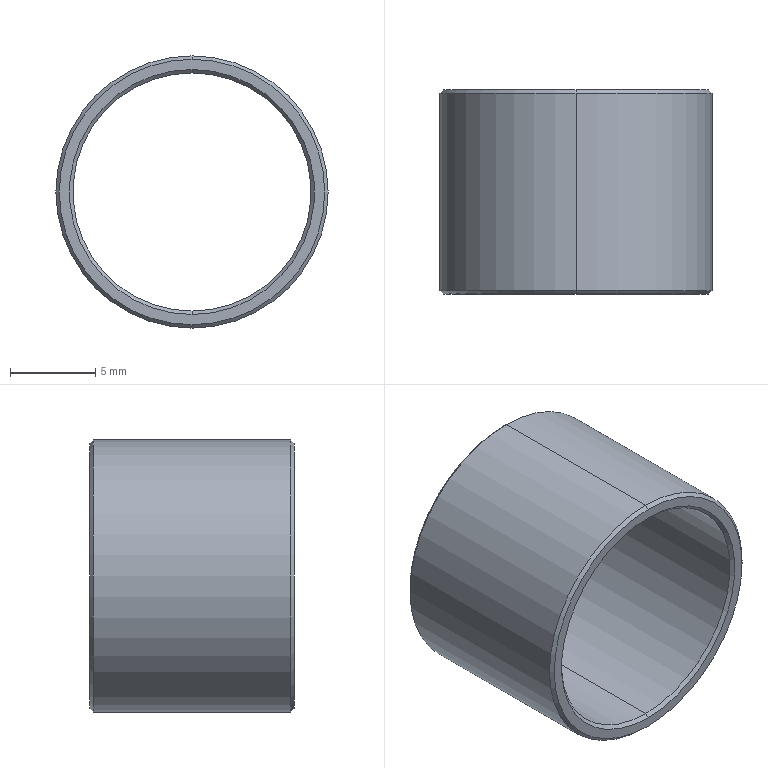Part | STEP file | Lead screw shaft end spacer V1.201001 | 1 solid | 14 faces | box 16 x 12 x 16 mm | volume 561.717 mm3 | cone 8 | cylinder 4 | plane 2 | commonest cylinder face diameters 14 x2 16 x2
STEP:
#1=CARTESIAN_POINT('',(0.,0.,0.));
#2=DIRECTION('',(0.,0.,1.));
#3=DIRECTION('',(1.,0.,0.));
#4=AXIS2_PLACEMENT_3D('',#1,#2,#3);
#5=CARTESIAN_POINT('',(0.,11.8,7.));
#6=VERTEX_POINT('',#5);
#7=CARTESIAN_POINT('',(0.,12.,7.2));
#8=VERTEX_POINT('',#7);
#9=CARTESIAN_POINT('',(0.,11.8,7.));
#10=DIRECTION('',(0.,0.7071,0.7071));
#11=VECTOR('',#10,1.);
#12=LINE('',#9,#11);
#13=CARTESIAN_POINT('',(0.,11.8,0.));
#14=DIRECTION('',(0.,1.,0.));
#15=DIRECTION('',(0.,0.,1.));
#16=AXIS2_PLACEMENT_3D('',#13,#14,#15);
#17=CONICAL_SURFACE('',#16,7.,0.7854);
#18=CARTESIAN_POINT('',(6.283,0.));
#19=DIRECTION('',(0.,1.));
#20=VECTOR('',#19,1.);
#21=LINE('',#18,#20);
#22=(GEOMETRIC_REPRESENTATION_CONTEXT(2)PARAMETRIC_REPRESENTATION_CONTEXT()REPRESENTATION_CONTEXT('',''));
#23=DEFINITIONAL_REPRESENTATION('',(#21),#22);
#24=PCURVE('',#17,#23);
#25=CARTESIAN_POINT('',(0.,11.8,0.));
#26=DIRECTION('',(0.,1.,0.));
#27=DIRECTION('',(0.,0.,1.));
#28=AXIS2_PLACEMENT_3D('',#25,#26,#27);
#29=CONICAL_SURFACE('',#28,7.,0.7854);
#30=CARTESIAN_POINT('',(0.,0.));
#31=DIRECTION('',(0.,1.));
#32=VECTOR('',#31,1.);
#33=LINE('',#30,#32);
#34=(GEOMETRIC_REPRESENTATION_CONTEXT(2)PARAMETRIC_REPRESENTATION_CONTEXT()REPRESENTATION_CONTEXT('',''));
#35=DEFINITIONAL_REPRESENTATION('',(#33),#34);
#36=PCURVE('',#29,#35);
#37=SURFACE_CURVE('',#12,(#24,#36),.PCURVE_S1.);
#38=EDGE_CURVE('',#6,#8,#37,.T.);
#39=ORIENTED_EDGE('',*,*,#38,.T.);
#40=CARTESIAN_POINT('',(0.,12.,-7.2));
#41=VERTEX_POINT('',#40);
#42=CARTESIAN_POINT('',(0.,12.,0.));
#43=DIRECTION('',(0.,-1.,0.));
#44=DIRECTION('',(0.,0.,1.));
#45=AXIS2_PLACEMENT_3D('',#42,#43,#44);
#46=CIRCLE('',#45,7.2);
#47=CARTESIAN_POINT('',(6.283,0.2));
#48=DIRECTION('',(-1.,0.));
#49=VECTOR('',#48,1.);
#50=LINE('',#47,#49);
#51=(GEOMETRIC_REPRESENTATION_CONTEXT(2)PARAMETRIC_REPRESENTATION_CONTEXT()REPRESENTATION_CONTEXT('',''));
#52=DEFINITIONAL_REPRESENTATION('',(#50),#51);
#53=PCURVE('',#17,#52);
#54=CARTESIAN_POINT('',(0.,12.,0.));
#55=DIRECTION('',(0.,1.,0.));
#56=DIRECTION('',(0.,0.,1.));
#57=AXIS2_PLACEMENT_3D('',#54,#55,#56);
#58=PLANE('',#57);
#59=CARTESIAN_POINT('',(7.2,0.));
#60=CARTESIAN_POINT('',(7.2,-12.471));
#61=CARTESIAN_POINT('',(-3.6,-6.235));
#62=CARTESIAN_POINT('',(-14.4,0.));
#63=CARTESIAN_POINT('',(-3.6,6.235));
#64=CARTESIAN_POINT('',(7.2,12.471));
#65=CARTESIAN_POINT('',(7.2,0.));
#66=(BOUNDED_CURVE()B_SPLINE_CURVE(2,(#59,#60,#61,#62,#63,#64,#65),.UNSPECIFIED.,.T.,.F.)B_SPLINE_CURVE_WITH_KNOTS((1,2,2,2,2,1),(-2.094,0.,2.094,4.189,6.283,8.378),.UNSPECIFIED.)CURVE()GEOMETRIC_REPRESENTATION_ITEM()RATIONAL_B_SPLINE_CURVE((1.,0.5,1.,0.5,1.,0.5,1.))REPRESENTATION_ITEM(''));
#67=(GEOMETRIC_REPRESENTATION_CONTEXT(2)PARAMETRIC_REPRESENTATION_CONTEXT()REPRESENTATION_CONTEXT('',''));
#68=DEFINITIONAL_REPRESENTATION('',(#66),#67);
#69=PCURVE('',#58,#68);
#70=SURFACE_CURVE('',#46,(#53,#69),.PCURVE_S1.);
#71=EDGE_CURVE('',#8,#41,#70,.T.);
#72=ORIENTED_EDGE('',*,*,#71,.T.);
#73=CARTESIAN_POINT('',(0.,11.8,-7.));
#74=VERTEX_POINT('',#73);
#75=CARTESIAN_POINT('',(0.,11.8,-7.));
#76=DIRECTION('',(0.,0.7071,-0.7071));
#77=VECTOR('',#76,1.);
#78=LINE('',#75,#77);
#79=CARTESIAN_POINT('',(3.142,0.));
#80=DIRECTION('',(0.,1.));
#81=VECTOR('',#80,1.);
#82=LINE('',#79,#81);
#83=(GEOMETRIC_REPRESENTATION_CONTEXT(2)PARAMETRIC_REPRESENTATION_CONTEXT()REPRESENTATION_CONTEXT('',''));
#84=DEFINITIONAL_REPRESENTATION('',(#82),#83);
#85=PCURVE('',#17,#84);
#86=CARTESIAN_POINT('',(3.142,0.));
#87=DIRECTION('',(0.,1.));
#88=VECTOR('',#87,1.);
#89=LINE('',#86,#88);
#90=(GEOMETRIC_REPRESENTATION_CONTEXT(2)PARAMETRIC_REPRESENTATION_CONTEXT()REPRESENTATION_CONTEXT('',''));
#91=DEFINITIONAL_REPRESENTATION('',(#89),#90);
#92=PCURVE('',#29,#91);
#93=SURFACE_CURVE('',#78,(#85,#92),.PCURVE_S1.);
#94=EDGE_CURVE('',#74,#41,#93,.T.);
#95=ORIENTED_EDGE('',*,*,#94,.F.);
#96=CARTESIAN_POINT('',(0.,11.8,0.));
#97=DIRECTION('',(0.,1.,0.));
#98=DIRECTION('',(0.,0.,1.));
#99=AXIS2_PLACEMENT_3D('',#96,#97,#98);
#100=CIRCLE('',#99,7.);
#101=CARTESIAN_POINT('',(0.,0.));
#102=DIRECTION('',(1.,0.));
#103=VECTOR('',#102,1.);
#104=LINE('',#101,#103);
#105=(GEOMETRIC_REPRESENTATION_CONTEXT(2)PARAMETRIC_REPRESENTATION_CONTEXT()REPRESENTATION_CONTEXT('',''));
#106=DEFINITIONAL_REPRESENTATION('',(#104),#105);
#107=PCURVE('',#17,#106);
#108=CARTESIAN_POINT('',(0.,12.,0.));
#109=DIRECTION('',(0.,-1.,0.));
#110=DIRECTION('',(0.,0.,-1.));
#111=AXIS2_PLACEMENT_3D('',#108,#109,#110);
#112=CYLINDRICAL_SURFACE('',#111,7.);
#113=CARTESIAN_POINT('',(9.425,0.2));
#114=DIRECTION('',(-1.,0.));
#115=VECTOR('',#114,1.);
#116=LINE('',#113,#115);
#117=(GEOMETRIC_REPRESENTATION_CONTEXT(2)PARAMETRIC_REPRESENTATION_CONTEXT()REPRESENTATION_CONTEXT('',''));
#118=DEFINITIONAL_REPRESENTATION('',(#116),#117);
#119=PCURVE('',#112,#118);
#120=SURFACE_CURVE('',#100,(#107,#119),.PCURVE_S1.);
#121=EDGE_CURVE('',#74,#6,#120,.T.);
#122=ORIENTED_EDGE('',*,*,#121,.T.);
#123=EDGE_LOOP('',(#39,#72,#95,#122));
#124=FACE_BOUND('',#123,.F.);
#125=ADVANCED_FACE('',(#124),#17,.F.);
#126=CARTESIAN_POINT('',(0.,12.,7.8));
#127=VERTEX_POINT('',#126);
#128=CARTESIAN_POINT('',(0.,12.,-7.8));
#129=VERTEX_POINT('',#128);
#130=CARTESIAN_POINT('',(0.,12.,0.));
#131=DIRECTION('',(0.,1.,0.));
#132=DIRECTION('',(0.,0.,1.));
#133=AXIS2_PLACEMENT_3D('',#130,#131,#132);
#134=CIRCLE('',#133,7.8);
#135=CARTESIAN_POINT('',(0.,12.,0.));
#136=DIRECTION('',(0.,-1.,0.));
#137=DIRECTION('',(0.,0.,-1.));
#138=AXIS2_PLACEMENT_3D('',#135,#136,#137);
#139=CONICAL_SURFACE('',#138,7.8,0.7854);
#140=CARTESIAN_POINT('',(3.142,0.));
#141=DIRECTION('',(-1.,0.));
#142=VECTOR('',#141,1.);
#143=LINE('',#140,#142);
#144=(GEOMETRIC_REPRESENTATION_CONTEXT(2)PARAMETRIC_REPRESENTATION_CONTEXT()REPRESENTATION_CONTEXT('',''));
#145=DEFINITIONAL_REPRESENTATION('',(#143),#144);
#146=PCURVE('',#139,#145);
#147=CARTESIAN_POINT('',(0.,0.));
#148=DIRECTION('',(1.,0.));
#149=AXIS2_PLACEMENT_2D('',#147,#148);
#150=CIRCLE('',#149,7.8);
#151=(GEOMETRIC_REPRESENTATION_CONTEXT(2)PARAMETRIC_REPRESENTATION_CONTEXT()REPRESENTATION_CONTEXT('',''));
#152=DEFINITIONAL_REPRESENTATION('',(#150),#151);
#153=PCURVE('',#58,#152);
#154=SURFACE_CURVE('',#134,(#146,#153),.PCURVE_S1.);
#155=EDGE_CURVE('',#127,#129,#154,.T.);
#156=ORIENTED_EDGE('',*,*,#155,.F.);
#157=CARTESIAN_POINT('',(0.,11.8,8.));
#158=VERTEX_POINT('',#157);
#159=CARTESIAN_POINT('',(0.,12.,7.8));
#160=DIRECTION('',(0.,-0.7071,0.7071));
#161=VECTOR('',#160,1.);
#162=LINE('',#159,#161);
#163=CARTESIAN_POINT('',(3.142,0.));
#164=DIRECTION('',(0.,1.));
#165=VECTOR('',#164,1.);
#166=LINE('',#163,#165);
#167=(GEOMETRIC_REPRESENTATION_CONTEXT(2)PARAMETRIC_REPRESENTATION_CONTEXT()REPRESENTATION_CONTEXT('',''));
#168=DEFINITIONAL_REPRESENTATION('',(#166),#167);
#169=PCURVE('',#139,#168);
#170=CARTESIAN_POINT('',(0.,12.,0.));
#171=DIRECTION('',(0.,-1.,0.));
#172=DIRECTION('',(0.,0.,-1.));
#173=AXIS2_PLACEMENT_3D('',#170,#171,#172);
#174=CONICAL_SURFACE('',#173,7.8,0.7854);
#175=CARTESIAN_POINT('',(3.142,0.));
#176=DIRECTION('',(0.,1.));
#177=VECTOR('',#176,1.);
#178=LINE('',#175,#177);
#179=(GEOMETRIC_REPRESENTATION_CONTEXT(2)PARAMETRIC_REPRESENTATION_CONTEXT()REPRESENTATION_CONTEXT('',''));
#180=DEFINITIONAL_REPRESENTATION('',(#178),#179);
#181=PCURVE('',#174,#180);
#182=SURFACE_CURVE('',#162,(#169,#181),.PCURVE_S1.);
#183=EDGE_CURVE('',#127,#158,#182,.T.);
#184=ORIENTED_EDGE('',*,*,#183,.T.);
#185=CARTESIAN_POINT('',(0.,11.8,-8.));
#186=VERTEX_POINT('',#185);
#187=CARTESIAN_POINT('',(0.,11.8,0.));
#188=DIRECTION('',(0.,-1.,0.));
#189=DIRECTION('',(0.,0.,1.));
#190=AXIS2_PLACEMENT_3D('',#187,#188,#189);
#191=CIRCLE('',#190,8.);
#192=CARTESIAN_POINT('',(-3.142,0.2));
#193=DIRECTION('',(1.,0.));
#194=VECTOR('',#193,1.);
#195=LINE('',#192,#194);
#196=(GEOMETRIC_REPRESENTATION_CONTEXT(2)PARAMETRIC_REPRESENTATION_CONTEXT()REPRESENTATION_CONTEXT('',''));
#197=DEFINITIONAL_REPRESENTATION('',(#195),#196);
#198=PCURVE('',#139,#197);
#199=CARTESIAN_POINT('',(0.,12.,0.));
#200=DIRECTION('',(0.,-1.,0.));
#201=DIRECTION('',(0.,0.,-1.));
#202=AXIS2_PLACEMENT_3D('',#199,#200,#201);
#203=CYLINDRICAL_SURFACE('',#202,8.);
#204=CARTESIAN_POINT('',(-3.142,0.2));
#205=DIRECTION('',(1.,0.));
#206=VECTOR('',#205,1.);
#207=LINE('',#204,#206);
#208=(GEOMETRIC_REPRESENTATION_CONTEXT(2)PARAMETRIC_REPRESENTATION_CONTEXT()REPRESENTATION_CONTEXT('',''));
#209=DEFINITIONAL_REPRESENTATION('',(#207),#208);
#210=PCURVE('',#203,#209);
#211=SURFACE_CURVE('',#191,(#198,#210),.PCURVE_S1.);
#212=EDGE_CURVE('',#186,#158,#211,.T.);
#213=ORIENTED_EDGE('',*,*,#212,.F.);
#214=CARTESIAN_POINT('',(0.,12.,-7.8));
#215=DIRECTION('',(0.,-0.7071,-0.7071));
#216=VECTOR('',#215,1.);
#217=LINE('',#214,#216);
#218=CARTESIAN_POINT('',(0.,0.));
#219=DIRECTION('',(0.,1.));
#220=VECTOR('',#219,1.);
#221=LINE('',#218,#220);
#222=(GEOMETRIC_REPRESENTATION_CONTEXT(2)PARAMETRIC_REPRESENTATION_CONTEXT()REPRESENTATION_CONTEXT('',''));
#223=DEFINITIONAL_REPRESENTATION('',(#221),#222);
#224=PCURVE('',#139,#223);
#225=CARTESIAN_POINT('',(6.283,0.));
#226=DIRECTION('',(0.,1.));
#227=VECTOR('',#226,1.);
#228=LINE('',#225,#227);
#229=(GEOMETRIC_REPRESENTATION_CONTEXT(2)PARAMETRIC_REPRESENTATION_CONTEXT()REPRESENTATION_CONTEXT('',''));
#230=DEFINITIONAL_REPRESENTATION('',(#228),#229);
#231=PCURVE('',#174,#230);
#232=SURFACE_CURVE('',#217,(#224,#231),.PCURVE_S1.);
#233=EDGE_CURVE('',#129,#186,#232,.T.);
#234=ORIENTED_EDGE('',*,*,#233,.F.);
#235=EDGE_LOOP('',(#156,#184,#213,#234));
#236=FACE_BOUND('',#235,.T.);
#237=ADVANCED_FACE('',(#236),#139,.T.);
#238=CARTESIAN_POINT('',(0.,0.,-7.8));
#239=VERTEX_POINT('',#238);
#240=CARTESIAN_POINT('',(0.,0.,7.8));
#241=VERTEX_POINT('',#240);
#242=CARTESIAN_POINT('',(0.,0.,0.));
#243=DIRECTION('',(0.,-1.,0.));
#244=DIRECTION('',(0.,0.,1.));
#245=AXIS2_PLACEMENT_3D('',#242,#243,#244);
#246=CIRCLE('',#245,7.8);
#247=CARTESIAN_POINT('',(0.,0.2,0.));
#248=DIRECTION('',(0.,1.,0.));
#249=DIRECTION('',(0.,0.,1.));
#250=AXIS2_PLACEMENT_3D('',#247,#248,#249);
#251=CONICAL_SURFACE('',#250,8.,0.7854);
#252=CARTESIAN_POINT('',(6.283,-0.2));
#253=DIRECTION('',(-1.,0.));
#254=VECTOR('',#253,1.);
#255=LINE('',#252,#254);
#256=(GEOMETRIC_REPRESENTATION_CONTEXT(2)PARAMETRIC_REPRESENTATION_CONTEXT()REPRESENTATION_CONTEXT('',''));
#257=DEFINITIONAL_REPRESENTATION('',(#255),#256);
#258=PCURVE('',#251,#257);
#259=CARTESIAN_POINT('',(0.,0.,0.));
#260=DIRECTION('',(0.,1.,0.));
#261=DIRECTION('',(0.,0.,1.));
#262=AXIS2_PLACEMENT_3D('',#259,#260,#261);
#263=PLANE('',#262);
#264=CARTESIAN_POINT('',(7.8,0.));
#265=CARTESIAN_POINT('',(7.8,-13.51));
#266=CARTESIAN_POINT('',(-3.9,-6.755));
#267=CARTESIAN_POINT('',(-15.6,0.));
#268=CARTESIAN_POINT('',(-3.9,6.755));
#269=CARTESIAN_POINT('',(7.8,13.51));
#270=CARTESIAN_POINT('',(7.8,0.));
#271=(BOUNDED_CURVE()B_SPLINE_CURVE(2,(#264,#265,#266,#267,#268,#269,#270),.UNSPECIFIED.,.T.,.F.)B_SPLINE_CURVE_WITH_KNOTS((1,2,2,2,2,1),(-2.094,0.,2.094,4.189,6.283,8.378),.UNSPECIFIED.)CURVE()GEOMETRIC_REPRESENTATION_ITEM()RATIONAL_B_SPLINE_CURVE((1.,0.5,1.,0.5,1.,0.5,1.))REPRESENTATION_ITEM(''));
#272=(GEOMETRIC_REPRESENTATION_CONTEXT(2)PARAMETRIC_REPRESENTATION_CONTEXT()REPRESENTATION_CONTEXT('',''));
#273=DEFINITIONAL_REPRESENTATION('',(#271),#272);
#274=PCURVE('',#263,#273);
#275=SURFACE_CURVE('',#246,(#258,#274),.PCURVE_S1.);
#276=EDGE_CURVE('',#239,#241,#275,.T.);
#277=ORIENTED_EDGE('',*,*,#276,.F.);
#278=CARTESIAN_POINT('',(0.,0.2,-8.));
#279=VERTEX_POINT('',#278);
#280=CARTESIAN_POINT('',(0.,0.2,-8.));
#281=DIRECTION('',(0.,0.7071,-0.7071));
#282=VECTOR('',#281,1.);
#283=LINE('',#280,#282);
#284=CARTESIAN_POINT('',(3.142,0.));
#285=DIRECTION('',(0.,1.));
#286=VECTOR('',#285,1.);
#287=LINE('',#284,#286);
#288=(GEOMETRIC_REPRESENTATION_CONTEXT(2)PARAMETRIC_REPRESENTATION_CONTEXT()REPRESENTATION_CONTEXT('',''));
#289=DEFINITIONAL_REPRESENTATION('',(#287),#288);
#290=PCURVE('',#251,#289);
#291=CARTESIAN_POINT('',(0.,0.2,0.));
#292=DIRECTION('',(0.,1.,0.));
#293=DIRECTION('',(0.,0.,1.));
#294=AXIS2_PLACEMENT_3D('',#291,#292,#293);
#295=CONICAL_SURFACE('',#294,8.,0.7854);
#296=CARTESIAN_POINT('',(3.142,0.));
#297=DIRECTION('',(0.,1.));
#298=VECTOR('',#297,1.);
#299=LINE('',#296,#298);
#300=(GEOMETRIC_REPRESENTATION_CONTEXT(2)PARAMETRIC_REPRESENTATION_CONTEXT()REPRESENTATION_CONTEXT('',''));
#301=DEFINITIONAL_REPRESENTATION('',(#299),#300);
#302=PCURVE('',#295,#301);
#303=SURFACE_CURVE('',#283,(#290,#302),.PCURVE_S1.);
#304=EDGE_CURVE('',#239,#279,#303,.T.);
#305=ORIENTED_EDGE('',*,*,#304,.T.);
#306=CARTESIAN_POINT('',(0.,0.2,8.));
#307=VERTEX_POINT('',#306);
#308=CARTESIAN_POINT('',(0.,0.2,0.));
#309=DIRECTION('',(0.,1.,0.));
#310=DIRECTION('',(0.,0.,1.));
#311=AXIS2_PLACEMENT_3D('',#308,#309,#310);
#312=CIRCLE('',#311,8.);
#313=CARTESIAN_POINT('',(0.,0.));
#314=DIRECTION('',(1.,0.));
#315=VECTOR('',#314,1.);
#316=LINE('',#313,#315);
#317=(GEOMETRIC_REPRESENTATION_CONTEXT(2)PARAMETRIC_REPRESENTATION_CONTEXT()REPRESENTATION_CONTEXT('',''));
#318=DEFINITIONAL_REPRESENTATION('',(#316),#317);
#319=PCURVE('',#251,#318);
#320=CARTESIAN_POINT('',(3.142,11.8));
#321=DIRECTION('',(-1.,0.));
#322=VECTOR('',#321,1.);
#323=LINE('',#320,#322);
#324=(GEOMETRIC_REPRESENTATION_CONTEXT(2)PARAMETRIC_REPRESENTATION_CONTEXT()REPRESENTATION_CONTEXT('',''));
#325=DEFINITIONAL_REPRESENTATION('',(#323),#324);
#326=PCURVE('',#203,#325);
#327=SURFACE_CURVE('',#312,(#319,#326),.PCURVE_S1.);
#328=EDGE_CURVE('',#307,#279,#327,.T.);
#329=ORIENTED_EDGE('',*,*,#328,.F.);
#330=CARTESIAN_POINT('',(0.,0.2,8.));
#331=DIRECTION('',(0.,0.7071,0.7071));
#332=VECTOR('',#331,1.);
#333=LINE('',#330,#332);
#334=CARTESIAN_POINT('',(0.,0.));
#335=DIRECTION('',(0.,1.));
#336=VECTOR('',#335,1.);
#337=LINE('',#334,#336);
#338=(GEOMETRIC_REPRESENTATION_CONTEXT(2)PARAMETRIC_REPRESENTATION_CONTEXT()REPRESENTATION_CONTEXT('',''));
#339=DEFINITIONAL_REPRESENTATION('',(#337),#338);
#340=PCURVE('',#251,#339);
#341=CARTESIAN_POINT('',(6.283,0.));
#342=DIRECTION('',(0.,1.));
#343=VECTOR('',#342,1.);
#344=LINE('',#341,#343);
#345=(GEOMETRIC_REPRESENTATION_CONTEXT(2)PARAMETRIC_REPRESENTATION_CONTEXT()REPRESENTATION_CONTEXT('',''));
#346=DEFINITIONAL_REPRESENTATION('',(#344),#345);
#347=PCURVE('',#295,#346);
#348=SURFACE_CURVE('',#333,(#340,#347),.PCURVE_S1.);
#349=EDGE_CURVE('',#241,#307,#348,.T.);
#350=ORIENTED_EDGE('',*,*,#349,.F.);
#351=EDGE_LOOP('',(#277,#305,#329,#350));
#352=FACE_BOUND('',#351,.T.);
#353=ADVANCED_FACE('',(#352),#251,.T.);
#354=CARTESIAN_POINT('',(0.,0.2,-7.));
#355=VERTEX_POINT('',#354);
#356=CARTESIAN_POINT('',(0.,0.,-7.2));
#357=VERTEX_POINT('',#356);
#358=CARTESIAN_POINT('',(0.,0.,-7.2));
#359=DIRECTION('',(0.,-0.7071,-0.7071));
#360=VECTOR('',#359,1.);
#361=LINE('',#358,#360);
#362=CARTESIAN_POINT('',(0.,0.,0.));
#363=DIRECTION('',(0.,-1.,0.));
#364=DIRECTION('',(0.,0.,-1.));
#365=AXIS2_PLACEMENT_3D('',#362,#363,#364);
#366=CONICAL_SURFACE('',#365,7.2,0.7854);
#367=CARTESIAN_POINT('',(6.283,0.));
#368=DIRECTION('',(0.,1.));
#369=VECTOR('',#368,1.);
#370=LINE('',#367,#369);
#371=(GEOMETRIC_REPRESENTATION_CONTEXT(2)PARAMETRIC_REPRESENTATION_CONTEXT()REPRESENTATION_CONTEXT('',''));
#372=DEFINITIONAL_REPRESENTATION('',(#370),#371);
#373=PCURVE('',#366,#372);
#374=CARTESIAN_POINT('',(0.,0.,0.));
#375=DIRECTION('',(0.,-1.,0.));
#376=DIRECTION('',(0.,0.,-1.));
#377=AXIS2_PLACEMENT_3D('',#374,#375,#376);
#378=CONICAL_SURFACE('',#377,7.2,0.7854);
#379=CARTESIAN_POINT('',(0.,0.));
#380=DIRECTION('',(0.,1.));
#381=VECTOR('',#380,1.);
#382=LINE('',#379,#381);
#383=(GEOMETRIC_REPRESENTATION_CONTEXT(2)PARAMETRIC_REPRESENTATION_CONTEXT()REPRESENTATION_CONTEXT('',''));
#384=DEFINITIONAL_REPRESENTATION('',(#382),#383);
#385=PCURVE('',#378,#384);
#386=SURFACE_CURVE('',#361,(#373,#385),.PCURVE_S1.);
#387=EDGE_CURVE('',#355,#357,#386,.T.);
#388=ORIENTED_EDGE('',*,*,#387,.T.);
#389=CARTESIAN_POINT('',(0.,0.,7.2));
#390=VERTEX_POINT('',#389);
#391=CARTESIAN_POINT('',(0.,0.,0.));
#392=DIRECTION('',(0.,1.,0.));
#393=DIRECTION('',(0.,0.,1.));
#394=AXIS2_PLACEMENT_3D('',#391,#392,#393);
#395=CIRCLE('',#394,7.2);
#396=CARTESIAN_POINT('',(9.425,0.));
#397=DIRECTION('',(-1.,0.));
#398=VECTOR('',#397,1.);
#399=LINE('',#396,#398);
#400=(GEOMETRIC_REPRESENTATION_CONTEXT(2)PARAMETRIC_REPRESENTATION_CONTEXT()REPRESENTATION_CONTEXT('',''));
#401=DEFINITIONAL_REPRESENTATION('',(#399),#400);
#402=PCURVE('',#366,#401);
#403=CARTESIAN_POINT('',(0.,0.));
#404=DIRECTION('',(1.,0.));
#405=AXIS2_PLACEMENT_2D('',#403,#404);
#406=CIRCLE('',#405,7.2);
#407=(GEOMETRIC_REPRESENTATION_CONTEXT(2)PARAMETRIC_REPRESENTATION_CONTEXT()REPRESENTATION_CONTEXT('',''));
#408=DEFINITIONAL_REPRESENTATION('',(#406),#407);
#409=PCURVE('',#263,#408);
#410=SURFACE_CURVE('',#395,(#402,#409),.PCURVE_S1.);
#411=EDGE_CURVE('',#357,#390,#410,.T.);
#412=ORIENTED_EDGE('',*,*,#411,.T.);
#413=CARTESIAN_POINT('',(0.,0.2,7.));
#414=VERTEX_POINT('',#413);
#415=CARTESIAN_POINT('',(0.,0.,7.2));
#416=DIRECTION('',(0.,-0.7071,0.7071));
#417=VECTOR('',#416,1.);
#418=LINE('',#415,#417);
#419=CARTESIAN_POINT('',(3.142,0.));
#420=DIRECTION('',(0.,1.));
#421=VECTOR('',#420,1.);
#422=LINE('',#419,#421);
#423=(GEOMETRIC_REPRESENTATION_CONTEXT(2)PARAMETRIC_REPRESENTATION_CONTEXT()REPRESENTATION_CONTEXT('',''));
#424=DEFINITIONAL_REPRESENTATION('',(#422),#423);
#425=PCURVE('',#366,#424);
#426=CARTESIAN_POINT('',(3.142,0.));
#427=DIRECTION('',(0.,1.));
#428=VECTOR('',#427,1.);
#429=LINE('',#426,#428);
#430=(GEOMETRIC_REPRESENTATION_CONTEXT(2)PARAMETRIC_REPRESENTATION_CONTEXT()REPRESENTATION_CONTEXT('',''));
#431=DEFINITIONAL_REPRESENTATION('',(#429),#430);
#432=PCURVE('',#378,#431);
#433=SURFACE_CURVE('',#418,(#425,#432),.PCURVE_S1.);
#434=EDGE_CURVE('',#414,#390,#433,.T.);
#435=ORIENTED_EDGE('',*,*,#434,.F.);
#436=CARTESIAN_POINT('',(0.,0.2,0.));
#437=DIRECTION('',(0.,-1.,0.));
#438=DIRECTION('',(0.,0.,1.));
#439=AXIS2_PLACEMENT_3D('',#436,#437,#438);
#440=CIRCLE('',#439,7.);
#441=CARTESIAN_POINT('',(3.142,-0.2));
#442=DIRECTION('',(1.,0.));
#443=VECTOR('',#442,1.);
#444=LINE('',#441,#443);
#445=(GEOMETRIC_REPRESENTATION_CONTEXT(2)PARAMETRIC_REPRESENTATION_CONTEXT()REPRESENTATION_CONTEXT('',''));
#446=DEFINITIONAL_REPRESENTATION('',(#444),#445);
#447=PCURVE('',#366,#446);
#448=CARTESIAN_POINT('',(3.142,11.8));
#449=DIRECTION('',(1.,0.));
#450=VECTOR('',#449,1.);
#451=LINE('',#448,#450);
#452=(GEOMETRIC_REPRESENTATION_CONTEXT(2)PARAMETRIC_REPRESENTATION_CONTEXT()REPRESENTATION_CONTEXT('',''));
#453=DEFINITIONAL_REPRESENTATION('',(#451),#452);
#454=PCURVE('',#112,#453);
#455=SURFACE_CURVE('',#440,(#447,#454),.PCURVE_S1.);
#456=EDGE_CURVE('',#414,#355,#455,.T.);
#457=ORIENTED_EDGE('',*,*,#456,.T.);
#458=EDGE_LOOP('',(#388,#412,#435,#457));
#459=FACE_BOUND('',#458,.F.);
#460=ADVANCED_FACE('',(#459),#366,.F.);
#461=CARTESIAN_POINT('',(0.,12.,-7.));
#462=DIRECTION('',(0.,-1.,0.));
#463=VECTOR('',#462,1.);
#464=LINE('',#461,#463);
#465=CARTESIAN_POINT('',(6.283,0.));
#466=DIRECTION('',(0.,1.));
#467=VECTOR('',#466,1.);
#468=LINE('',#465,#467);
#469=(GEOMETRIC_REPRESENTATION_CONTEXT(2)PARAMETRIC_REPRESENTATION_CONTEXT()REPRESENTATION_CONTEXT('',''));
#470=DEFINITIONAL_REPRESENTATION('',(#468),#469);
#471=PCURVE('',#112,#470);
#472=CARTESIAN_POINT('',(0.,12.,0.));
#473=DIRECTION('',(0.,-1.,0.));
#474=DIRECTION('',(0.,0.,-1.));
#475=AXIS2_PLACEMENT_3D('',#472,#473,#474);
#476=CYLINDRICAL_SURFACE('',#475,7.);
#477=CARTESIAN_POINT('',(0.,0.));
#478=DIRECTION('',(0.,1.));
#479=VECTOR('',#478,1.);
#480=LINE('',#477,#479);
#481=(GEOMETRIC_REPRESENTATION_CONTEXT(2)PARAMETRIC_REPRESENTATION_CONTEXT()REPRESENTATION_CONTEXT('',''));
#482=DEFINITIONAL_REPRESENTATION('',(#480),#481);
#483=PCURVE('',#476,#482);
#484=SURFACE_CURVE('',#464,(#471,#483),.PCURVE_S1.);
#485=EDGE_CURVE('',#74,#355,#484,.T.);
#486=ORIENTED_EDGE('',*,*,#485,.T.);
#487=ORIENTED_EDGE('',*,*,#456,.F.);
#488=CARTESIAN_POINT('',(0.,12.,7.));
#489=DIRECTION('',(0.,-1.,0.));
#490=VECTOR('',#489,1.);
#491=LINE('',#488,#490);
#492=CARTESIAN_POINT('',(3.142,0.));
#493=DIRECTION('',(0.,1.));
#494=VECTOR('',#493,1.);
#495=LINE('',#492,#494);
#496=(GEOMETRIC_REPRESENTATION_CONTEXT(2)PARAMETRIC_REPRESENTATION_CONTEXT()REPRESENTATION_CONTEXT('',''));
#497=DEFINITIONAL_REPRESENTATION('',(#495),#496);
#498=PCURVE('',#112,#497);
#499=CARTESIAN_POINT('',(3.142,0.));
#500=DIRECTION('',(0.,1.));
#501=VECTOR('',#500,1.);
#502=LINE('',#499,#501);
#503=(GEOMETRIC_REPRESENTATION_CONTEXT(2)PARAMETRIC_REPRESENTATION_CONTEXT()REPRESENTATION_CONTEXT('',''));
#504=DEFINITIONAL_REPRESENTATION('',(#502),#503);
#505=PCURVE('',#476,#504);
#506=SURFACE_CURVE('',#491,(#498,#505),.PCURVE_S1.);
#507=EDGE_CURVE('',#6,#414,#506,.T.);
#508=ORIENTED_EDGE('',*,*,#507,.F.);
#509=ORIENTED_EDGE('',*,*,#121,.F.);
#510=EDGE_LOOP('',(#486,#487,#508,#509));
#511=FACE_BOUND('',#510,.F.);
#512=ADVANCED_FACE('',(#511),#112,.F.);
#513=ORIENTED_EDGE('',*,*,#212,.T.);
#514=CARTESIAN_POINT('',(0.,12.,8.));
#515=DIRECTION('',(0.,-1.,0.));
#516=VECTOR('',#515,1.);
#517=LINE('',#514,#516);
#518=CARTESIAN_POINT('',(3.142,0.));
#519=DIRECTION('',(0.,1.));
#520=VECTOR('',#519,1.);
#521=LINE('',#518,#520);
#522=(GEOMETRIC_REPRESENTATION_CONTEXT(2)PARAMETRIC_REPRESENTATION_CONTEXT()REPRESENTATION_CONTEXT('',''));
#523=DEFINITIONAL_REPRESENTATION('',(#521),#522);
#524=PCURVE('',#203,#523);
#525=CARTESIAN_POINT('',(0.,12.,0.));
#526=DIRECTION('',(0.,-1.,0.));
#527=DIRECTION('',(0.,0.,-1.));
#528=AXIS2_PLACEMENT_3D('',#525,#526,#527);
#529=CYLINDRICAL_SURFACE('',#528,8.);
#530=CARTESIAN_POINT('',(3.142,0.));
#531=DIRECTION('',(0.,1.));
#532=VECTOR('',#531,1.);
#533=LINE('',#530,#532);
#534=(GEOMETRIC_REPRESENTATION_CONTEXT(2)PARAMETRIC_REPRESENTATION_CONTEXT()REPRESENTATION_CONTEXT('',''));
#535=DEFINITIONAL_REPRESENTATION('',(#533),#534);
#536=PCURVE('',#529,#535);
#537=SURFACE_CURVE('',#517,(#524,#536),.PCURVE_S1.);
#538=EDGE_CURVE('',#158,#307,#537,.T.);
#539=ORIENTED_EDGE('',*,*,#538,.T.);
#540=ORIENTED_EDGE('',*,*,#328,.T.);
#541=CARTESIAN_POINT('',(0.,12.,-8.));
#542=DIRECTION('',(0.,-1.,0.));
#543=VECTOR('',#542,1.);
#544=LINE('',#541,#543);
#545=CARTESIAN_POINT('',(0.,0.));
#546=DIRECTION('',(0.,1.));
#547=VECTOR('',#546,1.);
#548=LINE('',#545,#547);
#549=(GEOMETRIC_REPRESENTATION_CONTEXT(2)PARAMETRIC_REPRESENTATION_CONTEXT()REPRESENTATION_CONTEXT('',''));
#550=DEFINITIONAL_REPRESENTATION('',(#548),#549);
#551=PCURVE('',#203,#550);
#552=CARTESIAN_POINT('',(6.283,0.));
#553=DIRECTION('',(0.,1.));
#554=VECTOR('',#553,1.);
#555=LINE('',#552,#554);
#556=(GEOMETRIC_REPRESENTATION_CONTEXT(2)PARAMETRIC_REPRESENTATION_CONTEXT()REPRESENTATION_CONTEXT('',''));
#557=DEFINITIONAL_REPRESENTATION('',(#555),#556);
#558=PCURVE('',#529,#557);
#559=SURFACE_CURVE('',#544,(#551,#558),.PCURVE_S1.);
#560=EDGE_CURVE('',#186,#279,#559,.T.);
#561=ORIENTED_EDGE('',*,*,#560,.F.);
#562=EDGE_LOOP('',(#513,#539,#540,#561));
#563=FACE_BOUND('',#562,.T.);
#564=ADVANCED_FACE('',(#563),#203,.T.);
#565=CARTESIAN_POINT('',(0.,12.,0.));
#566=DIRECTION('',(0.,1.,0.));
#567=DIRECTION('',(0.,0.,1.));
#568=AXIS2_PLACEMENT_3D('',#565,#566,#567);
#569=CIRCLE('',#568,7.8);
#570=CARTESIAN_POINT('',(0.,0.));
#571=DIRECTION('',(1.,0.));
#572=AXIS2_PLACEMENT_2D('',#570,#571);
#573=CIRCLE('',#572,7.8);
#574=(GEOMETRIC_REPRESENTATION_CONTEXT(2)PARAMETRIC_REPRESENTATION_CONTEXT()REPRESENTATION_CONTEXT('',''));
#575=DEFINITIONAL_REPRESENTATION('',(#573),#574);
#576=PCURVE('',#58,#575);
#577=CARTESIAN_POINT('',(9.425,0.));
#578=DIRECTION('',(-1.,0.));
#579=VECTOR('',#578,1.);
#580=LINE('',#577,#579);
#581=(GEOMETRIC_REPRESENTATION_CONTEXT(2)PARAMETRIC_REPRESENTATION_CONTEXT()REPRESENTATION_CONTEXT('',''));
#582=DEFINITIONAL_REPRESENTATION('',(#580),#581);
#583=PCURVE('',#174,#582);
#584=SURFACE_CURVE('',#569,(#576,#583),.PCURVE_S1.);
#585=EDGE_CURVE('',#129,#127,#584,.T.);
#586=ORIENTED_EDGE('',*,*,#585,.T.);
#587=ORIENTED_EDGE('',*,*,#155,.T.);
#588=EDGE_LOOP('',(#586,#587));
#589=FACE_BOUND('',#588,.T.);
#590=ORIENTED_EDGE('',*,*,#71,.T.);
#591=CARTESIAN_POINT('',(0.,12.,0.));
#592=DIRECTION('',(0.,-1.,0.));
#593=DIRECTION('',(0.,0.,1.));
#594=AXIS2_PLACEMENT_3D('',#591,#592,#593);
#595=CIRCLE('',#594,7.2);
#596=CARTESIAN_POINT('',(7.2,0.));
#597=CARTESIAN_POINT('',(7.2,-12.471));
#598=CARTESIAN_POINT('',(-3.6,-6.235));
#599=CARTESIAN_POINT('',(-14.4,0.));
#600=CARTESIAN_POINT('',(-3.6,6.235));
#601=CARTESIAN_POINT('',(7.2,12.471));
#602=CARTESIAN_POINT('',(7.2,0.));
#603=(BOUNDED_CURVE()B_SPLINE_CURVE(2,(#596,#597,#598,#599,#600,#601,#602),.UNSPECIFIED.,.T.,.F.)B_SPLINE_CURVE_WITH_KNOTS((1,2,2,2,2,1),(-2.094,0.,2.094,4.189,6.283,8.378),.UNSPECIFIED.)CURVE()GEOMETRIC_REPRESENTATION_ITEM()RATIONAL_B_SPLINE_CURVE((1.,0.5,1.,0.5,1.,0.5,1.))REPRESENTATION_ITEM(''));
#604=(GEOMETRIC_REPRESENTATION_CONTEXT(2)PARAMETRIC_REPRESENTATION_CONTEXT()REPRESENTATION_CONTEXT('',''));
#605=DEFINITIONAL_REPRESENTATION('',(#603),#604);
#606=PCURVE('',#58,#605);
#607=CARTESIAN_POINT('',(6.283,0.2));
#608=DIRECTION('',(-1.,0.));
#609=VECTOR('',#608,1.);
#610=LINE('',#607,#609);
#611=(GEOMETRIC_REPRESENTATION_CONTEXT(2)PARAMETRIC_REPRESENTATION_CONTEXT()REPRESENTATION_CONTEXT('',''));
#612=DEFINITIONAL_REPRESENTATION('',(#610),#611);
#613=PCURVE('',#29,#612);
#614=SURFACE_CURVE('',#595,(#606,#613),.PCURVE_S1.);
#615=EDGE_CURVE('',#41,#8,#614,.T.);
#616=ORIENTED_EDGE('',*,*,#615,.T.);
#617=EDGE_LOOP('',(#590,#616));
#618=FACE_BOUND('',#617,.T.);
#619=ADVANCED_FACE('',(#589,#618),#58,.T.);
#620=ORIENTED_EDGE('',*,*,#411,.T.);
#621=CARTESIAN_POINT('',(0.,0.,0.));
#622=DIRECTION('',(0.,1.,0.));
#623=DIRECTION('',(0.,0.,1.));
#624=AXIS2_PLACEMENT_3D('',#621,#622,#623);
#625=CIRCLE('',#624,7.2);
#626=CARTESIAN_POINT('',(0.,0.));
#627=DIRECTION('',(1.,0.));
#628=AXIS2_PLACEMENT_2D('',#626,#627);
#629=CIRCLE('',#628,7.2);
#630=(GEOMETRIC_REPRESENTATION_CONTEXT(2)PARAMETRIC_REPRESENTATION_CONTEXT()REPRESENTATION_CONTEXT('',''));
#631=DEFINITIONAL_REPRESENTATION('',(#629),#630);
#632=PCURVE('',#263,#631);
#633=CARTESIAN_POINT('',(3.142,0.));
#634=DIRECTION('',(-1.,0.));
#635=VECTOR('',#634,1.);
#636=LINE('',#633,#635);
#637=(GEOMETRIC_REPRESENTATION_CONTEXT(2)PARAMETRIC_REPRESENTATION_CONTEXT()REPRESENTATION_CONTEXT('',''));
#638=DEFINITIONAL_REPRESENTATION('',(#636),#637);
#639=PCURVE('',#378,#638);
#640=SURFACE_CURVE('',#625,(#632,#639),.PCURVE_S1.);
#641=EDGE_CURVE('',#390,#357,#640,.T.);
#642=ORIENTED_EDGE('',*,*,#641,.T.);
#643=EDGE_LOOP('',(#620,#642));
#644=FACE_BOUND('',#643,.T.);
#645=CARTESIAN_POINT('',(0.,0.,0.));
#646=DIRECTION('',(0.,-1.,0.));
#647=DIRECTION('',(0.,0.,1.));
#648=AXIS2_PLACEMENT_3D('',#645,#646,#647);
#649=CIRCLE('',#648,7.8);
#650=CARTESIAN_POINT('',(7.8,0.));
#651=CARTESIAN_POINT('',(7.8,-13.51));
#652=CARTESIAN_POINT('',(-3.9,-6.755));
#653=CARTESIAN_POINT('',(-15.6,0.));
#654=CARTESIAN_POINT('',(-3.9,6.755));
#655=CARTESIAN_POINT('',(7.8,13.51));
#656=CARTESIAN_POINT('',(7.8,0.));
#657=(BOUNDED_CURVE()B_SPLINE_CURVE(2,(#650,#651,#652,#653,#654,#655,#656),.UNSPECIFIED.,.T.,.F.)B_SPLINE_CURVE_WITH_KNOTS((1,2,2,2,2,1),(-2.094,0.,2.094,4.189,6.283,8.378),.UNSPECIFIED.)CURVE()GEOMETRIC_REPRESENTATION_ITEM()RATIONAL_B_SPLINE_CURVE((1.,0.5,1.,0.5,1.,0.5,1.))REPRESENTATION_ITEM(''));
#658=(GEOMETRIC_REPRESENTATION_CONTEXT(2)PARAMETRIC_REPRESENTATION_CONTEXT()REPRESENTATION_CONTEXT('',''));
#659=DEFINITIONAL_REPRESENTATION('',(#657),#658);
#660=PCURVE('',#263,#659);
#661=CARTESIAN_POINT('',(6.283,-0.2));
#662=DIRECTION('',(-1.,0.));
#663=VECTOR('',#662,1.);
#664=LINE('',#661,#663);
#665=(GEOMETRIC_REPRESENTATION_CONTEXT(2)PARAMETRIC_REPRESENTATION_CONTEXT()REPRESENTATION_CONTEXT('',''));
#666=DEFINITIONAL_REPRESENTATION('',(#664),#665);
#667=PCURVE('',#295,#666);
#668=SURFACE_CURVE('',#649,(#660,#667),.PCURVE_S1.);
#669=EDGE_CURVE('',#241,#239,#668,.T.);
#670=ORIENTED_EDGE('',*,*,#669,.T.);
#671=ORIENTED_EDGE('',*,*,#276,.T.);
#672=EDGE_LOOP('',(#670,#671));
#673=FACE_BOUND('',#672,.T.);
#674=ADVANCED_FACE('',(#644,#673),#263,.F.);
#675=ORIENTED_EDGE('',*,*,#538,.F.);
#676=CARTESIAN_POINT('',(0.,11.8,0.));
#677=DIRECTION('',(0.,-1.,0.));
#678=DIRECTION('',(0.,0.,1.));
#679=AXIS2_PLACEMENT_3D('',#676,#677,#678);
#680=CIRCLE('',#679,8.);
#681=CARTESIAN_POINT('',(3.142,0.2));
#682=DIRECTION('',(1.,0.));
#683=VECTOR('',#682,1.);
#684=LINE('',#681,#683);
#685=(GEOMETRIC_REPRESENTATION_CONTEXT(2)PARAMETRIC_REPRESENTATION_CONTEXT()REPRESENTATION_CONTEXT('',''));
#686=DEFINITIONAL_REPRESENTATION('',(#684),#685);
#687=PCURVE('',#529,#686);
#688=CARTESIAN_POINT('',(3.142,0.2));
#689=DIRECTION('',(1.,0.));
#690=VECTOR('',#689,1.);
#691=LINE('',#688,#690);
#692=(GEOMETRIC_REPRESENTATION_CONTEXT(2)PARAMETRIC_REPRESENTATION_CONTEXT()REPRESENTATION_CONTEXT('',''));
#693=DEFINITIONAL_REPRESENTATION('',(#691),#692);
#694=PCURVE('',#174,#693);
#695=SURFACE_CURVE('',#680,(#687,#694),.PCURVE_S1.);
#696=EDGE_CURVE('',#158,#186,#695,.T.);
#697=ORIENTED_EDGE('',*,*,#696,.T.);
#698=ORIENTED_EDGE('',*,*,#560,.T.);
#699=CARTESIAN_POINT('',(0.,0.2,0.));
#700=DIRECTION('',(0.,1.,0.));
#701=DIRECTION('',(0.,0.,1.));
#702=AXIS2_PLACEMENT_3D('',#699,#700,#701);
#703=CIRCLE('',#702,8.);
#704=CARTESIAN_POINT('',(9.425,11.8));
#705=DIRECTION('',(-1.,0.));
#706=VECTOR('',#705,1.);
#707=LINE('',#704,#706);
#708=(GEOMETRIC_REPRESENTATION_CONTEXT(2)PARAMETRIC_REPRESENTATION_CONTEXT()REPRESENTATION_CONTEXT('',''));
#709=DEFINITIONAL_REPRESENTATION('',(#707),#708);
#710=PCURVE('',#529,#709);
#711=CARTESIAN_POINT('',(0.,0.));
#712=DIRECTION('',(1.,0.));
#713=VECTOR('',#712,1.);
#714=LINE('',#711,#713);
#715=(GEOMETRIC_REPRESENTATION_CONTEXT(2)PARAMETRIC_REPRESENTATION_CONTEXT()REPRESENTATION_CONTEXT('',''));
#716=DEFINITIONAL_REPRESENTATION('',(#714),#715);
#717=PCURVE('',#295,#716);
#718=SURFACE_CURVE('',#703,(#710,#717),.PCURVE_S1.);
#719=EDGE_CURVE('',#279,#307,#718,.T.);
#720=ORIENTED_EDGE('',*,*,#719,.T.);
#721=EDGE_LOOP('',(#675,#697,#698,#720));
#722=FACE_BOUND('',#721,.T.);
#723=ADVANCED_FACE('',(#722),#529,.T.);
#724=CARTESIAN_POINT('',(0.,0.2,0.));
#725=DIRECTION('',(0.,-1.,0.));
#726=DIRECTION('',(0.,0.,1.));
#727=AXIS2_PLACEMENT_3D('',#724,#725,#726);
#728=CIRCLE('',#727,7.);
#729=CARTESIAN_POINT('',(-3.142,11.8));
#730=DIRECTION('',(1.,0.));
#731=VECTOR('',#730,1.);
#732=LINE('',#729,#731);
#733=(GEOMETRIC_REPRESENTATION_CONTEXT(2)PARAMETRIC_REPRESENTATION_CONTEXT()REPRESENTATION_CONTEXT('',''));
#734=DEFINITIONAL_REPRESENTATION('',(#732),#733);
#735=PCURVE('',#476,#734);
#736=CARTESIAN_POINT('',(-3.142,-0.2));
#737=DIRECTION('',(1.,0.));
#738=VECTOR('',#737,1.);
#739=LINE('',#736,#738);
#740=(GEOMETRIC_REPRESENTATION_CONTEXT(2)PARAMETRIC_REPRESENTATION_CONTEXT()REPRESENTATION_CONTEXT('',''));
#741=DEFINITIONAL_REPRESENTATION('',(#739),#740);
#742=PCURVE('',#378,#741);
#743=SURFACE_CURVE('',#728,(#735,#742),.PCURVE_S1.);
#744=EDGE_CURVE('',#355,#414,#743,.T.);
#745=ORIENTED_EDGE('',*,*,#744,.F.);
#746=ORIENTED_EDGE('',*,*,#485,.F.);
#747=CARTESIAN_POINT('',(0.,11.8,0.));
#748=DIRECTION('',(0.,1.,0.));
#749=DIRECTION('',(0.,0.,1.));
#750=AXIS2_PLACEMENT_3D('',#747,#748,#749);
#751=CIRCLE('',#750,7.);
#752=CARTESIAN_POINT('',(3.142,0.2));
#753=DIRECTION('',(-1.,0.));
#754=VECTOR('',#753,1.);
#755=LINE('',#752,#754);
#756=(GEOMETRIC_REPRESENTATION_CONTEXT(2)PARAMETRIC_REPRESENTATION_CONTEXT()REPRESENTATION_CONTEXT('',''));
#757=DEFINITIONAL_REPRESENTATION('',(#755),#756);
#758=PCURVE('',#476,#757);
#759=CARTESIAN_POINT('',(0.,0.));
#760=DIRECTION('',(1.,0.));
#761=VECTOR('',#760,1.);
#762=LINE('',#759,#761);
#763=(GEOMETRIC_REPRESENTATION_CONTEXT(2)PARAMETRIC_REPRESENTATION_CONTEXT()REPRESENTATION_CONTEXT('',''));
#764=DEFINITIONAL_REPRESENTATION('',(#762),#763);
#765=PCURVE('',#29,#764);
#766=SURFACE_CURVE('',#751,(#758,#765),.PCURVE_S1.);
#767=EDGE_CURVE('',#6,#74,#766,.T.);
#768=ORIENTED_EDGE('',*,*,#767,.F.);
#769=ORIENTED_EDGE('',*,*,#507,.T.);
#770=EDGE_LOOP('',(#745,#746,#768,#769));
#771=FACE_BOUND('',#770,.F.);
#772=ADVANCED_FACE('',(#771),#476,.F.);
#773=ORIENTED_EDGE('',*,*,#641,.T.);
#774=ORIENTED_EDGE('',*,*,#387,.F.);
#775=ORIENTED_EDGE('',*,*,#744,.T.);
#776=ORIENTED_EDGE('',*,*,#434,.T.);
#777=EDGE_LOOP('',(#773,#774,#775,#776));
#778=FACE_BOUND('',#777,.F.);
#779=ADVANCED_FACE('',(#778),#378,.F.);
#780=ORIENTED_EDGE('',*,*,#304,.F.);
#781=ORIENTED_EDGE('',*,*,#669,.F.);
#782=ORIENTED_EDGE('',*,*,#349,.T.);
#783=ORIENTED_EDGE('',*,*,#719,.F.);
#784=EDGE_LOOP('',(#780,#781,#782,#783));
#785=FACE_BOUND('',#784,.T.);
#786=ADVANCED_FACE('',(#785),#295,.T.);
#787=ORIENTED_EDGE('',*,*,#183,.F.);
#788=ORIENTED_EDGE('',*,*,#585,.F.);
#789=ORIENTED_EDGE('',*,*,#233,.T.);
#790=ORIENTED_EDGE('',*,*,#696,.F.);
#791=EDGE_LOOP('',(#787,#788,#789,#790));
#792=FACE_BOUND('',#791,.T.);
#793=ADVANCED_FACE('',(#792),#174,.T.);
#794=ORIENTED_EDGE('',*,*,#615,.T.);
#795=ORIENTED_EDGE('',*,*,#38,.F.);
#796=ORIENTED_EDGE('',*,*,#767,.T.);
#797=ORIENTED_EDGE('',*,*,#94,.T.);
#798=EDGE_LOOP('',(#794,#795,#796,#797));
#799=FACE_BOUND('',#798,.F.);
#800=ADVANCED_FACE('',(#799),#29,.F.);
#801=CLOSED_SHELL('',(#125,#237,#353,#460,#512,#564,#619,#674,#723,#772,#779,#786,#793,#800));
#802=MANIFOLD_SOLID_BREP('',#801);
#803=(LENGTH_UNIT()NAMED_UNIT(*)SI_UNIT(.MILLI.,.METRE.));
#804=UNCERTAINTY_MEASURE_WITH_UNIT(LENGTH_MEASURE(0.0000001),#803,'','');
#805=(NAMED_UNIT(*)PLANE_ANGLE_UNIT()SI_UNIT($,.RADIAN.));
#806=(NAMED_UNIT(*)SI_UNIT($,.STERADIAN.)SOLID_ANGLE_UNIT());
#807=(GEOMETRIC_REPRESENTATION_CONTEXT(3)GLOBAL_UNCERTAINTY_ASSIGNED_CONTEXT((#804))GLOBAL_UNIT_ASSIGNED_CONTEXT((#803,#805,#806))REPRESENTATION_CONTEXT('',''));
#808=ADVANCED_BREP_SHAPE_REPRESENTATION('',(#4,#802),#807);